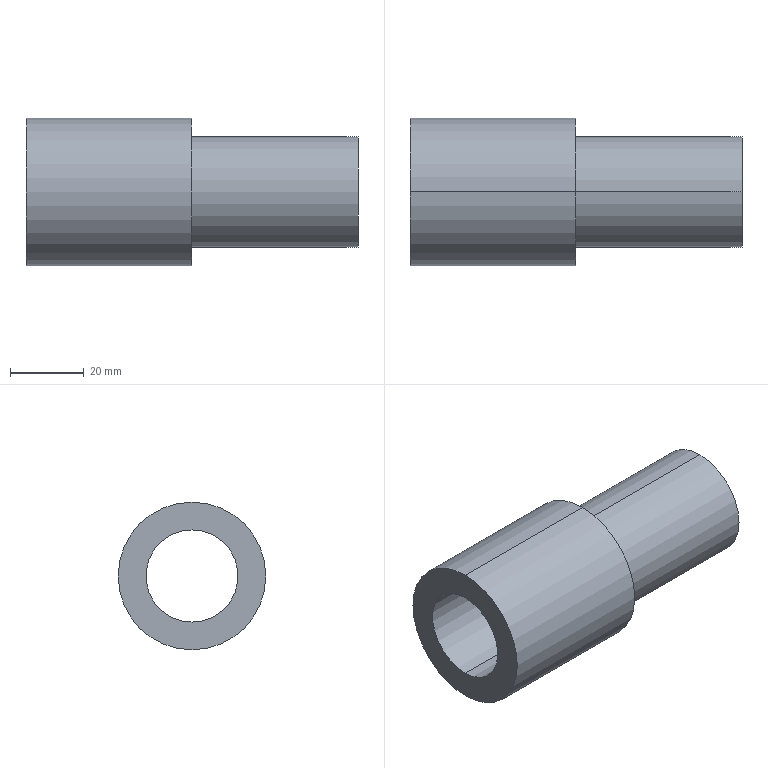Part | SolidWorks | features ICE 1, RefAxis 1, Revolution 1 | 1 solid | 9 faces | box 90 x 40 x 40 mm | volume 44179 mm3 | cylinder 6 | plane 3 | commonest cylinder face diameters 25 x2 30 x2 40 x2
STEP:
#1=CARTESIAN_POINT('',(0.,0.,-12.5));
#2=VERTEX_POINT('',#1);
#3=CARTESIAN_POINT('',(0.,0.,12.5));
#4=VERTEX_POINT('',#3);
#5=CARTESIAN_POINT('',(0.,0.,0.));
#6=DIRECTION('',(-1.,0.,0.));
#7=DIRECTION('',(0.,0.,-1.));
#8=AXIS2_PLACEMENT_3D('',#5,#6,#7);
#9=CIRCLE('',#8,12.5);
#10=EDGE_CURVE('',#2,#4,#9,.T.);
#11=ORIENTED_EDGE('',*,*,#10,.T.);
#12=CARTESIAN_POINT('',(90.,0.,12.5));
#13=VERTEX_POINT('',#12);
#14=CARTESIAN_POINT('',(-0.001,0.,12.5));
#15=DIRECTION('',(1.,0.,0.));
#16=VECTOR('',#15,1000.);
#17=LINE('',#14,#16);
#18=EDGE_CURVE('',#4,#13,#17,.T.);
#19=ORIENTED_EDGE('',*,*,#18,.T.);
#20=CARTESIAN_POINT('',(90.,0.,-12.5));
#21=VERTEX_POINT('',#20);
#22=CARTESIAN_POINT('',(90.,0.,0.));
#23=DIRECTION('',(1.,0.,0.));
#24=DIRECTION('',(0.,0.,-1.));
#25=AXIS2_PLACEMENT_3D('',#22,#23,#24);
#26=CIRCLE('',#25,12.5);
#27=EDGE_CURVE('',#13,#21,#26,.T.);
#28=ORIENTED_EDGE('',*,*,#27,.T.);
#29=CARTESIAN_POINT('',(-0.001,0.,-12.5));
#30=DIRECTION('',(1.,0.,0.));
#31=VECTOR('',#30,1000.);
#32=LINE('',#29,#31);
#33=EDGE_CURVE('',#2,#21,#32,.T.);
#34=ORIENTED_EDGE('',*,*,#33,.F.);
#35=EDGE_LOOP('',(#11,#19,#28,#34));
#36=FACE_OUTER_BOUND('',#35,.T.);
#37=CARTESIAN_POINT('',(-0.001,0.,0.));
#38=DIRECTION('',(1.,0.,0.));
#39=DIRECTION('',(0.,0.,-1.));
#40=AXIS2_PLACEMENT_3D('',#37,#38,#39);
#41=CYLINDRICAL_SURFACE('',#40,12.5);
#42=ADVANCED_FACE('',(#36),#41,.F.);
#43=CARTESIAN_POINT('',(90.,0.,15.));
#44=VERTEX_POINT('',#43);
#45=CARTESIAN_POINT('',(90.,0.,-15.));
#46=VERTEX_POINT('',#45);
#47=CARTESIAN_POINT('',(90.,0.,0.));
#48=DIRECTION('',(-1.,0.,0.));
#49=DIRECTION('',(0.,0.,1.));
#50=AXIS2_PLACEMENT_3D('',#47,#48,#49);
#51=CIRCLE('',#50,15.);
#52=EDGE_CURVE('',#44,#46,#51,.T.);
#53=ORIENTED_EDGE('',*,*,#52,.T.);
#54=CARTESIAN_POINT('',(45.,0.,-15.));
#55=VERTEX_POINT('',#54);
#56=CARTESIAN_POINT('',(-36.554,0.,-15.));
#57=DIRECTION('',(-1.,0.,0.));
#58=VECTOR('',#57,1000.);
#59=LINE('',#56,#58);
#60=EDGE_CURVE('',#46,#55,#59,.T.);
#61=ORIENTED_EDGE('',*,*,#60,.T.);
#62=CARTESIAN_POINT('',(45.,0.,15.));
#63=VERTEX_POINT('',#62);
#64=CARTESIAN_POINT('',(45.,0.,0.));
#65=DIRECTION('',(-1.,0.,0.));
#66=DIRECTION('',(0.,0.,1.));
#67=AXIS2_PLACEMENT_3D('',#64,#65,#66);
#68=CIRCLE('',#67,15.);
#69=EDGE_CURVE('',#63,#55,#68,.T.);
#70=ORIENTED_EDGE('',*,*,#69,.F.);
#71=CARTESIAN_POINT('',(-36.554,0.,15.));
#72=DIRECTION('',(-1.,0.,0.));
#73=VECTOR('',#72,1000.);
#74=LINE('',#71,#73);
#75=EDGE_CURVE('',#44,#63,#74,.T.);
#76=ORIENTED_EDGE('',*,*,#75,.F.);
#77=EDGE_LOOP('',(#53,#61,#70,#76));
#78=FACE_OUTER_BOUND('',#77,.T.);
#79=CARTESIAN_POINT('',(-36.554,0.,0.));
#80=DIRECTION('',(-1.,0.,0.));
#81=DIRECTION('',(0.,0.,1.));
#82=AXIS2_PLACEMENT_3D('',#79,#80,#81);
#83=CYLINDRICAL_SURFACE('',#82,15.);
#84=ADVANCED_FACE('',(#78),#83,.T.);
#85=CARTESIAN_POINT('',(45.,0.,20.));
#86=VERTEX_POINT('',#85);
#87=CARTESIAN_POINT('',(45.,0.,-20.));
#88=VERTEX_POINT('',#87);
#89=CARTESIAN_POINT('',(45.,0.,0.));
#90=DIRECTION('',(-1.,0.,0.));
#91=DIRECTION('',(0.,0.,1.));
#92=AXIS2_PLACEMENT_3D('',#89,#90,#91);
#93=CIRCLE('',#92,20.);
#94=EDGE_CURVE('',#86,#88,#93,.T.);
#95=ORIENTED_EDGE('',*,*,#94,.T.);
#96=CARTESIAN_POINT('',(0.,0.,-20.));
#97=VERTEX_POINT('',#96);
#98=CARTESIAN_POINT('',(-36.554,0.,-20.));
#99=DIRECTION('',(-1.,0.,0.));
#100=VECTOR('',#99,1000.);
#101=LINE('',#98,#100);
#102=EDGE_CURVE('',#88,#97,#101,.T.);
#103=ORIENTED_EDGE('',*,*,#102,.T.);
#104=CARTESIAN_POINT('',(0.,0.,20.));
#105=VERTEX_POINT('',#104);
#106=CARTESIAN_POINT('',(0.,0.,0.));
#107=DIRECTION('',(-1.,0.,0.));
#108=DIRECTION('',(0.,0.,1.));
#109=AXIS2_PLACEMENT_3D('',#106,#107,#108);
#110=CIRCLE('',#109,20.);
#111=EDGE_CURVE('',#105,#97,#110,.T.);
#112=ORIENTED_EDGE('',*,*,#111,.F.);
#113=CARTESIAN_POINT('',(-36.554,0.,20.));
#114=DIRECTION('',(-1.,0.,0.));
#115=VECTOR('',#114,1000.);
#116=LINE('',#113,#115);
#117=EDGE_CURVE('',#86,#105,#116,.T.);
#118=ORIENTED_EDGE('',*,*,#117,.F.);
#119=EDGE_LOOP('',(#95,#103,#112,#118));
#120=FACE_OUTER_BOUND('',#119,.T.);
#121=CARTESIAN_POINT('',(-36.554,0.,0.));
#122=DIRECTION('',(-1.,0.,0.));
#123=DIRECTION('',(0.,0.,1.));
#124=AXIS2_PLACEMENT_3D('',#121,#122,#123);
#125=CYLINDRICAL_SURFACE('',#124,20.);
#126=ADVANCED_FACE('',(#120),#125,.T.);
#127=ORIENTED_EDGE('',*,*,#10,.F.);
#128=CARTESIAN_POINT('',(0.,0.,0.));
#129=DIRECTION('',(-1.,0.,0.));
#130=DIRECTION('',(0.,0.,-1.));
#131=AXIS2_PLACEMENT_3D('',#128,#129,#130);
#132=CIRCLE('',#131,12.5);
#133=EDGE_CURVE('',#4,#2,#132,.T.);
#134=ORIENTED_EDGE('',*,*,#133,.F.);
#135=EDGE_LOOP('',(#127,#134));
#136=FACE_BOUND('',#135,.T.);
#137=ORIENTED_EDGE('',*,*,#111,.T.);
#138=CARTESIAN_POINT('',(0.,0.,0.));
#139=DIRECTION('',(-1.,0.,0.));
#140=DIRECTION('',(0.,0.,1.));
#141=AXIS2_PLACEMENT_3D('',#138,#139,#140);
#142=CIRCLE('',#141,20.);
#143=EDGE_CURVE('',#97,#105,#142,.T.);
#144=ORIENTED_EDGE('',*,*,#143,.T.);
#145=EDGE_LOOP('',(#137,#144));
#146=FACE_OUTER_BOUND('',#145,.T.);
#147=CARTESIAN_POINT('',(0.,0.,0.));
#148=DIRECTION('',(1.,0.,0.));
#149=DIRECTION('',(0.,0.,-1.));
#150=AXIS2_PLACEMENT_3D('',#147,#148,#149);
#151=PLANE('',#150);
#152=ADVANCED_FACE('',(#136,#146),#151,.F.);
#153=ORIENTED_EDGE('',*,*,#102,.F.);
#154=CARTESIAN_POINT('',(45.,0.,0.));
#155=DIRECTION('',(-1.,0.,0.));
#156=DIRECTION('',(0.,0.,1.));
#157=AXIS2_PLACEMENT_3D('',#154,#155,#156);
#158=CIRCLE('',#157,20.);
#159=EDGE_CURVE('',#88,#86,#158,.T.);
#160=ORIENTED_EDGE('',*,*,#159,.T.);
#161=ORIENTED_EDGE('',*,*,#117,.T.);
#162=ORIENTED_EDGE('',*,*,#143,.F.);
#163=EDGE_LOOP('',(#153,#160,#161,#162));
#164=FACE_OUTER_BOUND('',#163,.T.);
#165=CARTESIAN_POINT('',(-36.554,0.,0.));
#166=DIRECTION('',(-1.,0.,0.));
#167=DIRECTION('',(0.,0.,1.));
#168=AXIS2_PLACEMENT_3D('',#165,#166,#167);
#169=CYLINDRICAL_SURFACE('',#168,20.);
#170=ADVANCED_FACE('',(#164),#169,.T.);
#171=ORIENTED_EDGE('',*,*,#94,.F.);
#172=ORIENTED_EDGE('',*,*,#159,.F.);
#173=EDGE_LOOP('',(#171,#172));
#174=FACE_OUTER_BOUND('',#173,.T.);
#175=ORIENTED_EDGE('',*,*,#69,.T.);
#176=CARTESIAN_POINT('',(45.,0.,0.));
#177=DIRECTION('',(-1.,0.,0.));
#178=DIRECTION('',(0.,0.,1.));
#179=AXIS2_PLACEMENT_3D('',#176,#177,#178);
#180=CIRCLE('',#179,15.);
#181=EDGE_CURVE('',#55,#63,#180,.T.);
#182=ORIENTED_EDGE('',*,*,#181,.T.);
#183=EDGE_LOOP('',(#175,#182));
#184=FACE_BOUND('',#183,.T.);
#185=CARTESIAN_POINT('',(45.,20.,0.));
#186=DIRECTION('',(-1.,0.,0.));
#187=DIRECTION('',(0.,0.,1.));
#188=AXIS2_PLACEMENT_3D('',#185,#186,#187);
#189=PLANE('',#188);
#190=ADVANCED_FACE('',(#174,#184),#189,.F.);
#191=ORIENTED_EDGE('',*,*,#60,.F.);
#192=CARTESIAN_POINT('',(90.,0.,0.));
#193=DIRECTION('',(-1.,0.,0.));
#194=DIRECTION('',(0.,0.,1.));
#195=AXIS2_PLACEMENT_3D('',#192,#193,#194);
#196=CIRCLE('',#195,15.);
#197=EDGE_CURVE('',#46,#44,#196,.T.);
#198=ORIENTED_EDGE('',*,*,#197,.T.);
#199=ORIENTED_EDGE('',*,*,#75,.T.);
#200=ORIENTED_EDGE('',*,*,#181,.F.);
#201=EDGE_LOOP('',(#191,#198,#199,#200));
#202=FACE_OUTER_BOUND('',#201,.T.);
#203=CARTESIAN_POINT('',(-36.554,0.,0.));
#204=DIRECTION('',(-1.,0.,0.));
#205=DIRECTION('',(0.,0.,1.));
#206=AXIS2_PLACEMENT_3D('',#203,#204,#205);
#207=CYLINDRICAL_SURFACE('',#206,15.);
#208=ADVANCED_FACE('',(#202),#207,.T.);
#209=CARTESIAN_POINT('',(90.,0.,0.));
#210=DIRECTION('',(1.,0.,0.));
#211=DIRECTION('',(0.,0.,-1.));
#212=AXIS2_PLACEMENT_3D('',#209,#210,#211);
#213=CIRCLE('',#212,12.5);
#214=EDGE_CURVE('',#21,#13,#213,.T.);
#215=ORIENTED_EDGE('',*,*,#214,.F.);
#216=ORIENTED_EDGE('',*,*,#27,.F.);
#217=EDGE_LOOP('',(#215,#216));
#218=FACE_BOUND('',#217,.T.);
#219=ORIENTED_EDGE('',*,*,#52,.F.);
#220=ORIENTED_EDGE('',*,*,#197,.F.);
#221=EDGE_LOOP('',(#219,#220));
#222=FACE_OUTER_BOUND('',#221,.T.);
#223=CARTESIAN_POINT('',(90.,15.,0.));
#224=DIRECTION('',(-1.,0.,0.));
#225=DIRECTION('',(0.,0.,1.));
#226=AXIS2_PLACEMENT_3D('',#223,#224,#225);
#227=PLANE('',#226);
#228=ADVANCED_FACE('',(#218,#222),#227,.F.);
#229=ORIENTED_EDGE('',*,*,#18,.F.);
#230=ORIENTED_EDGE('',*,*,#133,.T.);
#231=ORIENTED_EDGE('',*,*,#33,.T.);
#232=ORIENTED_EDGE('',*,*,#214,.T.);
#233=EDGE_LOOP('',(#229,#230,#231,#232));
#234=FACE_OUTER_BOUND('',#233,.T.);
#235=CARTESIAN_POINT('',(-0.001,0.,0.));
#236=DIRECTION('',(1.,0.,0.));
#237=DIRECTION('',(0.,0.,-1.));
#238=AXIS2_PLACEMENT_3D('',#235,#236,#237);
#239=CYLINDRICAL_SURFACE('',#238,12.5);
#240=ADVANCED_FACE('',(#234),#239,.F.);
#241=CLOSED_SHELL('',(#42,#84,#126,#152,#170,#190,#208,#228,#240));
#242=MANIFOLD_SOLID_BREP('',#241);
#243=CARTESIAN_POINT('',(0.,0.,0.));
#244=DIRECTION('',(0.,0.,1.));
#245=DIRECTION('',(1.,0.,0.));
#246=AXIS2_PLACEMENT_3D('',#243,#244,#245);
#247=(LENGTH_UNIT()NAMED_UNIT(*)SI_UNIT(.MILLI.,.METRE.));
#248=UNCERTAINTY_MEASURE_WITH_UNIT(LENGTH_MEASURE(0.00001),#247,'','');
#249=(NAMED_UNIT(*)PLANE_ANGLE_UNIT()SI_UNIT($,.RADIAN.));
#250=(NAMED_UNIT(*)SI_UNIT($,.STERADIAN.)SOLID_ANGLE_UNIT());
#251=(GEOMETRIC_REPRESENTATION_CONTEXT(3)GLOBAL_UNCERTAINTY_ASSIGNED_CONTEXT((#248))GLOBAL_UNIT_ASSIGNED_CONTEXT((#247,#249,#250))REPRESENTATION_CONTEXT('',''));
#252=ADVANCED_BREP_SHAPE_REPRESENTATION('',(#242,#246),#251);